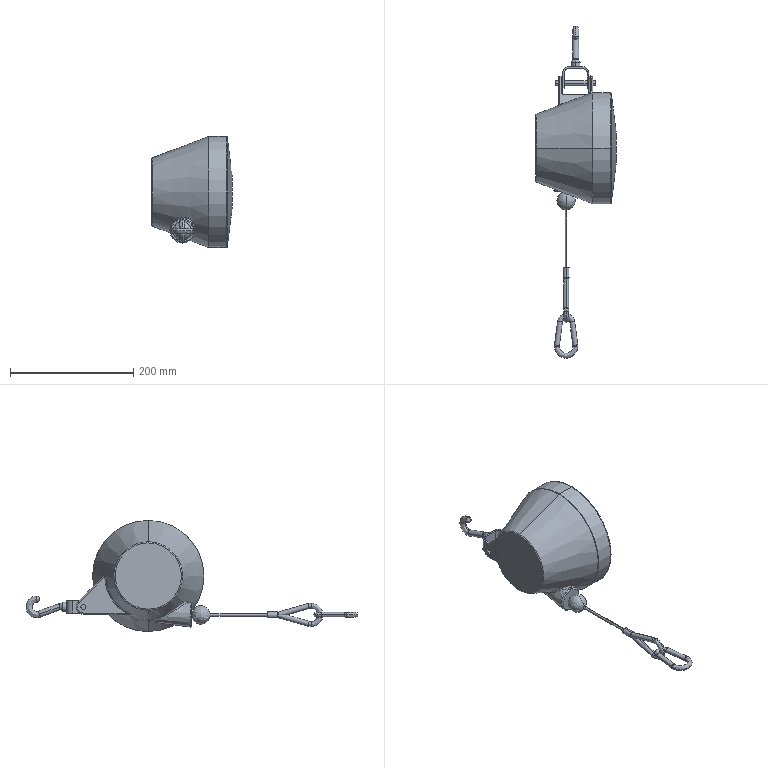Part | SolidWorks | features BaseBody 3 | 3 solids | 140 faces | box 130 x 538 x 180 mm | volume 2549222 mm3 | spline 62 | cylinder 43 | plane 27 | cone 8 | commonest cylinder face diameters 4 x16 8 x15 10 x2 14 x2 15 x2 20 x2